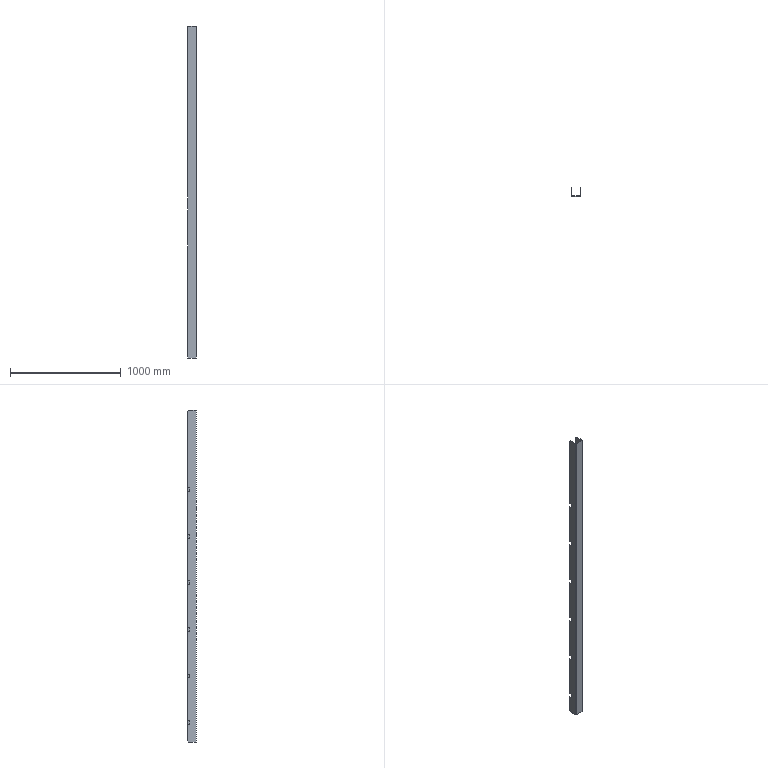Part | STEP file | SX-004-06 | 1 solid | 50 faces | box 80 x 80 x 2996 mm | volume 1398905 mm3 | plane 46 | cylinder 4 | commonest cylinder face diameters 0.4 x2 4.4 x2